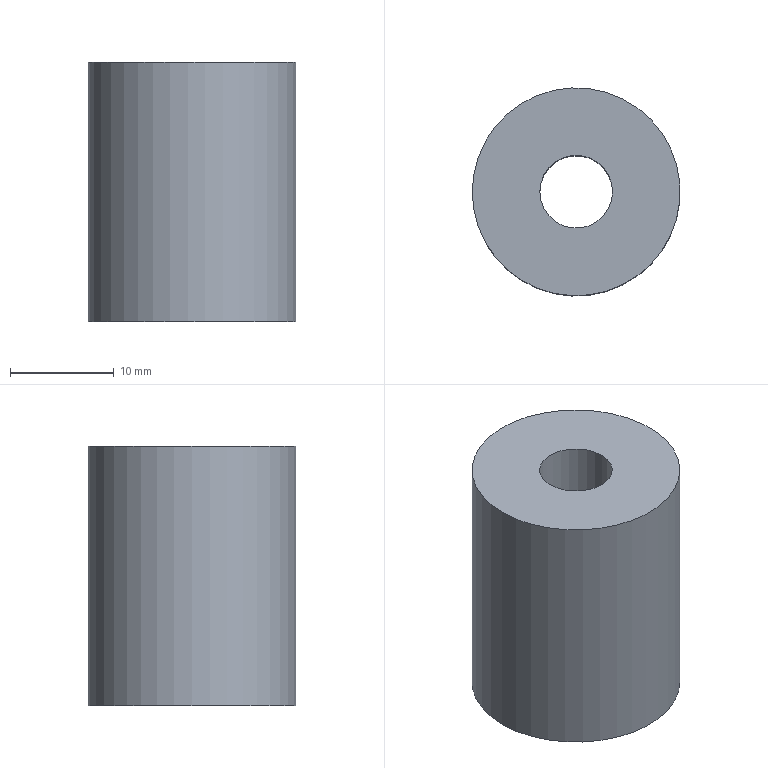Part | NX | features solid 2 | 1 solid | 4 faces | box 20 x 20 x 25 mm | volume 6892 mm3 | cylinder 2 | plane 2 | commonest cylinder face diameters 7 x1 20 x1
STEP:
#1=CARTESIAN_POINT('',(1524.116,80.895,-4.));
#2=VERTEX_POINT('',#1);
#3=CARTESIAN_POINT('',(1534.116,80.895,-4.));
#4=DIRECTION('',(0.,0.,-1.));
#5=DIRECTION('',(-1.,0.,0.));
#6=AXIS2_PLACEMENT_3D('',#3,#4,#5);
#7=CIRCLE('',#6,10.);
#8=EDGE_CURVE('',#2,#2,#7,.T.);
#9=ORIENTED_EDGE('',*,*,#8,.T.);
#10=EDGE_LOOP('',(#9));
#11=FACE_BOUND('',#10,.T.);
#12=CARTESIAN_POINT('',(1524.116,80.895,-29.));
#13=VERTEX_POINT('',#12);
#14=CARTESIAN_POINT('',(1534.116,80.895,-29.));
#15=DIRECTION('',(0.,0.,-1.));
#16=DIRECTION('',(-1.,0.,0.));
#17=AXIS2_PLACEMENT_3D('',#14,#15,#16);
#18=CIRCLE('',#17,10.);
#19=EDGE_CURVE('',#13,#13,#18,.T.);
#20=ORIENTED_EDGE('',*,*,#19,.F.);
#21=EDGE_LOOP('',(#20));
#22=FACE_BOUND('',#21,.T.);
#23=CARTESIAN_POINT('',(1534.116,80.895,-4.));
#24=DIRECTION('',(0.,0.,-1.));
#25=DIRECTION('',(1.,0.,0.));
#26=AXIS2_PLACEMENT_3D('',#23,#24,#25);
#27=CYLINDRICAL_SURFACE('',#26,10.);
#28=ADVANCED_FACE('',(#11,#22),#27,.T.);
#29=CARTESIAN_POINT('',(1530.616,80.895,-4.));
#30=VERTEX_POINT('',#29);
#31=CARTESIAN_POINT('',(1534.116,80.895,-4.));
#32=DIRECTION('',(0.,0.,-1.));
#33=DIRECTION('',(-1.,0.,0.));
#34=AXIS2_PLACEMENT_3D('',#31,#32,#33);
#35=CIRCLE('',#34,3.5);
#36=EDGE_CURVE('',#30,#30,#35,.T.);
#37=ORIENTED_EDGE('',*,*,#36,.T.);
#38=EDGE_LOOP('',(#37));
#39=FACE_BOUND('',#38,.T.);
#40=ORIENTED_EDGE('',*,*,#8,.F.);
#41=EDGE_LOOP('',(#40));
#42=FACE_BOUND('',#41,.T.);
#43=CARTESIAN_POINT('',(1534.116,80.895,-4.));
#44=DIRECTION('',(0.,0.,1.));
#45=DIRECTION('',(-1.,0.,0.));
#46=AXIS2_PLACEMENT_3D('',#43,#44,#45);
#47=PLANE('',#46);
#48=ADVANCED_FACE('',(#39,#42),#47,.T.);
#49=CARTESIAN_POINT('',(1530.616,80.895,-29.));
#50=VERTEX_POINT('',#49);
#51=CARTESIAN_POINT('',(1534.116,80.895,-29.));
#52=DIRECTION('',(0.,0.,-1.));
#53=DIRECTION('',(-1.,0.,0.));
#54=AXIS2_PLACEMENT_3D('',#51,#52,#53);
#55=CIRCLE('',#54,3.5);
#56=EDGE_CURVE('',#50,#50,#55,.T.);
#57=ORIENTED_EDGE('',*,*,#56,.F.);
#58=EDGE_LOOP('',(#57));
#59=FACE_BOUND('',#58,.T.);
#60=ORIENTED_EDGE('',*,*,#19,.T.);
#61=EDGE_LOOP('',(#60));
#62=FACE_BOUND('',#61,.T.);
#63=CARTESIAN_POINT('',(1534.116,80.895,-29.));
#64=DIRECTION('',(0.,0.,1.));
#65=DIRECTION('',(-1.,0.,0.));
#66=AXIS2_PLACEMENT_3D('',#63,#64,#65);
#67=PLANE('',#66);
#68=ADVANCED_FACE('',(#59,#62),#67,.F.);
#69=ORIENTED_EDGE('',*,*,#36,.F.);
#70=EDGE_LOOP('',(#69));
#71=FACE_BOUND('',#70,.T.);
#72=ORIENTED_EDGE('',*,*,#56,.T.);
#73=EDGE_LOOP('',(#72));
#74=FACE_BOUND('',#73,.T.);
#75=CARTESIAN_POINT('',(1534.116,80.895,-29.));
#76=DIRECTION('',(0.,0.,1.));
#77=DIRECTION('',(-1.,0.,0.));
#78=AXIS2_PLACEMENT_3D('',#75,#76,#77);
#79=CYLINDRICAL_SURFACE('',#78,3.5);
#80=ADVANCED_FACE('',(#71,#74),#79,.F.);
#81=CLOSED_SHELL('',(#28,#48,#68,#80));
#82=MANIFOLD_SOLID_BREP('',#81);
#83=(LENGTH_UNIT()NAMED_UNIT(*)SI_UNIT(.MILLI.,.METRE.));
#84=UNCERTAINTY_MEASURE_WITH_UNIT(LENGTH_MEASURE(0.00001),#83,'','');
#85=(NAMED_UNIT(*)PLANE_ANGLE_UNIT()SI_UNIT($,.RADIAN.));
#86=(NAMED_UNIT(*)SI_UNIT($,.STERADIAN.)SOLID_ANGLE_UNIT());
#87=(GEOMETRIC_REPRESENTATION_CONTEXT(3)GLOBAL_UNCERTAINTY_ASSIGNED_CONTEXT((#84))GLOBAL_UNIT_ASSIGNED_CONTEXT((#83,#85,#86))REPRESENTATION_CONTEXT('',''));
#88=ADVANCED_BREP_SHAPE_REPRESENTATION('',(#82),#87);